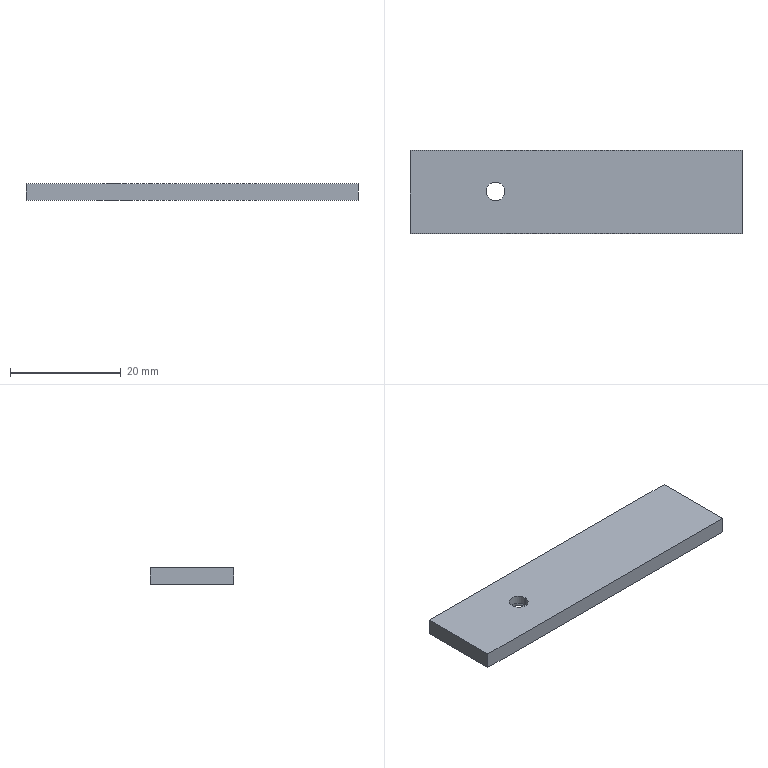Part | SolidWorks | features 3DProfileFeature 1, Extrusion 1, HoleWzd 1 | 1 solid | 10 faces | box 60 x 15 x 3 mm | volume 2658 mm3 | plane 6 | cone 2 | cylinder 2 | commonest cylinder face diameters 3.4 x2
STEP:
#1=CARTESIAN_POINT('',(-12.834,0.1148,1.45));
#2=VERTEX_POINT('',#1);
#3=CARTESIAN_POINT('',(-16.234,0.1148,1.45));
#4=VERTEX_POINT('',#3);
#5=CARTESIAN_POINT('',(-14.534,0.1148,1.45));
#6=DIRECTION('',(0.,0.,-1.));
#7=DIRECTION('',(-1.,0.,0.));
#8=AXIS2_PLACEMENT_3D('',#5,#6,#7);
#9=CIRCLE('',#8,1.7);
#10=EDGE_CURVE('',#2,#4,#9,.T.);
#11=ORIENTED_EDGE('',*,*,#10,.F.);
#12=CARTESIAN_POINT('',(-11.384,0.1148,0.));
#13=VERTEX_POINT('',#12);
#14=CARTESIAN_POINT('',(-11.384,0.1148,0.));
#15=DIRECTION('',(0.7071,0.,-0.7071));
#16=VECTOR('',#15,1000.);
#17=LINE('',#14,#16);
#18=EDGE_CURVE('',#2,#13,#17,.T.);
#19=ORIENTED_EDGE('',*,*,#18,.T.);
#20=CARTESIAN_POINT('',(-17.684,0.1148,0.));
#21=VERTEX_POINT('',#20);
#22=CARTESIAN_POINT('',(-14.534,0.1148,0.));
#23=DIRECTION('',(0.,0.,-1.));
#24=DIRECTION('',(-1.,0.,0.));
#25=AXIS2_PLACEMENT_3D('',#22,#23,#24);
#26=CIRCLE('',#25,3.15);
#27=EDGE_CURVE('',#13,#21,#26,.T.);
#28=ORIENTED_EDGE('',*,*,#27,.T.);
#29=CARTESIAN_POINT('',(-17.684,0.1148,0.));
#30=DIRECTION('',(-0.7071,0.,-0.7071));
#31=VECTOR('',#30,1000.);
#32=LINE('',#29,#31);
#33=EDGE_CURVE('',#4,#21,#32,.T.);
#34=ORIENTED_EDGE('',*,*,#33,.F.);
#35=EDGE_LOOP('',(#11,#19,#28,#34));
#36=FACE_OUTER_BOUND('',#35,.T.);
#37=CARTESIAN_POINT('',(-14.534,0.1148,0.));
#38=DIRECTION('',(0.,0.,-1.));
#39=DIRECTION('',(-1.,0.,0.));
#40=AXIS2_PLACEMENT_3D('',#37,#38,#39);
#41=CONICAL_SURFACE('',#40,3.15,0.7854);
#42=ADVANCED_FACE('',(#36),#41,.F.);
#43=CARTESIAN_POINT('',(-12.834,0.1148,3.));
#44=VERTEX_POINT('',#43);
#45=CARTESIAN_POINT('',(-16.234,0.1148,3.));
#46=VERTEX_POINT('',#45);
#47=CARTESIAN_POINT('',(-14.534,0.1148,3.));
#48=DIRECTION('',(0.,0.,-1.));
#49=DIRECTION('',(-1.,0.,0.));
#50=AXIS2_PLACEMENT_3D('',#47,#48,#49);
#51=CIRCLE('',#50,1.7);
#52=EDGE_CURVE('',#44,#46,#51,.T.);
#53=ORIENTED_EDGE('',*,*,#52,.F.);
#54=CARTESIAN_POINT('',(-12.834,0.1148,0.));
#55=DIRECTION('',(0.,0.,-1.));
#56=VECTOR('',#55,1000.);
#57=LINE('',#54,#56);
#58=EDGE_CURVE('',#44,#2,#57,.T.);
#59=ORIENTED_EDGE('',*,*,#58,.T.);
#60=ORIENTED_EDGE('',*,*,#10,.T.);
#61=CARTESIAN_POINT('',(-16.234,0.1148,0.));
#62=DIRECTION('',(0.,0.,-1.));
#63=VECTOR('',#62,1000.);
#64=LINE('',#61,#63);
#65=EDGE_CURVE('',#46,#4,#64,.T.);
#66=ORIENTED_EDGE('',*,*,#65,.F.);
#67=EDGE_LOOP('',(#53,#59,#60,#66));
#68=FACE_OUTER_BOUND('',#67,.T.);
#69=CARTESIAN_POINT('',(-14.534,0.1148,0.));
#70=DIRECTION('',(0.,0.,-1.));
#71=DIRECTION('',(-1.,0.,0.));
#72=AXIS2_PLACEMENT_3D('',#69,#70,#71);
#73=CYLINDRICAL_SURFACE('',#72,1.7);
#74=ADVANCED_FACE('',(#68),#73,.F.);
#75=CARTESIAN_POINT('',(30.,-7.5,0.));
#76=VERTEX_POINT('',#75);
#77=CARTESIAN_POINT('',(30.,7.5,0.));
#78=VERTEX_POINT('',#77);
#79=CARTESIAN_POINT('',(30.,-7.5,0.));
#80=DIRECTION('',(0.,1.,0.));
#81=VECTOR('',#80,1000.);
#82=LINE('',#79,#81);
#83=EDGE_CURVE('',#76,#78,#82,.T.);
#84=ORIENTED_EDGE('',*,*,#83,.T.);
#85=CARTESIAN_POINT('',(30.,7.5,3.));
#86=VERTEX_POINT('',#85);
#87=CARTESIAN_POINT('',(30.,7.5,3.));
#88=DIRECTION('',(0.,0.,-1.));
#89=VECTOR('',#88,1000.);
#90=LINE('',#87,#89);
#91=EDGE_CURVE('',#86,#78,#90,.T.);
#92=ORIENTED_EDGE('',*,*,#91,.F.);
#93=CARTESIAN_POINT('',(30.,-7.5,3.));
#94=VERTEX_POINT('',#93);
#95=CARTESIAN_POINT('',(30.,-7.5,3.));
#96=DIRECTION('',(0.,1.,0.));
#97=VECTOR('',#96,1000.);
#98=LINE('',#95,#97);
#99=EDGE_CURVE('',#94,#86,#98,.T.);
#100=ORIENTED_EDGE('',*,*,#99,.F.);
#101=CARTESIAN_POINT('',(30.,-7.5,3.));
#102=DIRECTION('',(0.,0.,-1.));
#103=VECTOR('',#102,1000.);
#104=LINE('',#101,#103);
#105=EDGE_CURVE('',#94,#76,#104,.T.);
#106=ORIENTED_EDGE('',*,*,#105,.T.);
#107=EDGE_LOOP('',(#84,#92,#100,#106));
#108=FACE_OUTER_BOUND('',#107,.T.);
#109=CARTESIAN_POINT('',(30.,-7.5,3.));
#110=DIRECTION('',(-1.,0.,0.));
#111=DIRECTION('',(0.,0.,1.));
#112=AXIS2_PLACEMENT_3D('',#109,#110,#111);
#113=PLANE('',#112);
#114=ADVANCED_FACE('',(#108),#113,.F.);
#115=CARTESIAN_POINT('',(-30.,7.5,0.));
#116=VERTEX_POINT('',#115);
#117=CARTESIAN_POINT('',(-30.,7.5,0.));
#118=DIRECTION('',(-1.,0.,0.));
#119=VECTOR('',#118,1000.);
#120=LINE('',#117,#119);
#121=EDGE_CURVE('',#78,#116,#120,.T.);
#122=ORIENTED_EDGE('',*,*,#121,.T.);
#123=CARTESIAN_POINT('',(-30.,7.5,3.));
#124=VERTEX_POINT('',#123);
#125=CARTESIAN_POINT('',(-30.,7.5,3.));
#126=DIRECTION('',(0.,0.,-1.));
#127=VECTOR('',#126,1000.);
#128=LINE('',#125,#127);
#129=EDGE_CURVE('',#124,#116,#128,.T.);
#130=ORIENTED_EDGE('',*,*,#129,.F.);
#131=CARTESIAN_POINT('',(-30.,7.5,3.));
#132=DIRECTION('',(-1.,0.,0.));
#133=VECTOR('',#132,1000.);
#134=LINE('',#131,#133);
#135=EDGE_CURVE('',#86,#124,#134,.T.);
#136=ORIENTED_EDGE('',*,*,#135,.F.);
#137=ORIENTED_EDGE('',*,*,#91,.T.);
#138=EDGE_LOOP('',(#122,#130,#136,#137));
#139=FACE_OUTER_BOUND('',#138,.T.);
#140=CARTESIAN_POINT('',(-30.,7.5,3.));
#141=DIRECTION('',(0.,-1.,0.));
#142=DIRECTION('',(0.,0.,-1.));
#143=AXIS2_PLACEMENT_3D('',#140,#141,#142);
#144=PLANE('',#143);
#145=ADVANCED_FACE('',(#139),#144,.F.);
#146=CARTESIAN_POINT('',(-30.,-7.5,0.));
#147=VERTEX_POINT('',#146);
#148=CARTESIAN_POINT('',(-30.,-7.5,0.));
#149=DIRECTION('',(0.,-1.,0.));
#150=VECTOR('',#149,1000.);
#151=LINE('',#148,#150);
#152=EDGE_CURVE('',#116,#147,#151,.T.);
#153=ORIENTED_EDGE('',*,*,#152,.T.);
#154=CARTESIAN_POINT('',(-30.,-7.5,3.));
#155=VERTEX_POINT('',#154);
#156=CARTESIAN_POINT('',(-30.,-7.5,3.));
#157=DIRECTION('',(0.,0.,-1.));
#158=VECTOR('',#157,1000.);
#159=LINE('',#156,#158);
#160=EDGE_CURVE('',#155,#147,#159,.T.);
#161=ORIENTED_EDGE('',*,*,#160,.F.);
#162=CARTESIAN_POINT('',(-30.,-7.5,3.));
#163=DIRECTION('',(0.,-1.,0.));
#164=VECTOR('',#163,1000.);
#165=LINE('',#162,#164);
#166=EDGE_CURVE('',#124,#155,#165,.T.);
#167=ORIENTED_EDGE('',*,*,#166,.F.);
#168=ORIENTED_EDGE('',*,*,#129,.T.);
#169=EDGE_LOOP('',(#153,#161,#167,#168));
#170=FACE_OUTER_BOUND('',#169,.T.);
#171=CARTESIAN_POINT('',(-30.,-7.5,3.));
#172=DIRECTION('',(1.,0.,0.));
#173=DIRECTION('',(0.,0.,-1.));
#174=AXIS2_PLACEMENT_3D('',#171,#172,#173);
#175=PLANE('',#174);
#176=ADVANCED_FACE('',(#170),#175,.F.);
#177=CARTESIAN_POINT('',(-30.,-7.5,0.));
#178=DIRECTION('',(1.,0.,0.));
#179=VECTOR('',#178,1000.);
#180=LINE('',#177,#179);
#181=EDGE_CURVE('',#147,#76,#180,.T.);
#182=ORIENTED_EDGE('',*,*,#181,.T.);
#183=ORIENTED_EDGE('',*,*,#105,.F.);
#184=CARTESIAN_POINT('',(-30.,-7.5,3.));
#185=DIRECTION('',(1.,0.,0.));
#186=VECTOR('',#185,1000.);
#187=LINE('',#184,#186);
#188=EDGE_CURVE('',#155,#94,#187,.T.);
#189=ORIENTED_EDGE('',*,*,#188,.F.);
#190=ORIENTED_EDGE('',*,*,#160,.T.);
#191=EDGE_LOOP('',(#182,#183,#189,#190));
#192=FACE_OUTER_BOUND('',#191,.T.);
#193=CARTESIAN_POINT('',(-30.,-7.5,3.));
#194=DIRECTION('',(0.,1.,0.));
#195=DIRECTION('',(0.,0.,1.));
#196=AXIS2_PLACEMENT_3D('',#193,#194,#195);
#197=PLANE('',#196);
#198=ADVANCED_FACE('',(#192),#197,.F.);
#199=CARTESIAN_POINT('',(-14.534,0.1148,3.));
#200=DIRECTION('',(0.,0.,-1.));
#201=DIRECTION('',(-1.,0.,0.));
#202=AXIS2_PLACEMENT_3D('',#199,#200,#201);
#203=CIRCLE('',#202,1.7);
#204=EDGE_CURVE('',#46,#44,#203,.T.);
#205=ORIENTED_EDGE('',*,*,#204,.T.);
#206=ORIENTED_EDGE('',*,*,#52,.T.);
#207=EDGE_LOOP('',(#205,#206));
#208=FACE_BOUND('',#207,.T.);
#209=ORIENTED_EDGE('',*,*,#99,.T.);
#210=ORIENTED_EDGE('',*,*,#135,.T.);
#211=ORIENTED_EDGE('',*,*,#166,.T.);
#212=ORIENTED_EDGE('',*,*,#188,.T.);
#213=EDGE_LOOP('',(#209,#210,#211,#212));
#214=FACE_OUTER_BOUND('',#213,.T.);
#215=CARTESIAN_POINT('',(0.,0.,3.));
#216=DIRECTION('',(0.,0.,-1.));
#217=DIRECTION('',(-1.,0.,0.));
#218=AXIS2_PLACEMENT_3D('',#215,#216,#217);
#219=PLANE('',#218);
#220=ADVANCED_FACE('',(#208,#214),#219,.F.);
#221=CARTESIAN_POINT('',(-14.534,0.1148,0.));
#222=DIRECTION('',(0.,0.,-1.));
#223=DIRECTION('',(-1.,0.,0.));
#224=AXIS2_PLACEMENT_3D('',#221,#222,#223);
#225=CIRCLE('',#224,3.15);
#226=EDGE_CURVE('',#21,#13,#225,.T.);
#227=ORIENTED_EDGE('',*,*,#226,.F.);
#228=ORIENTED_EDGE('',*,*,#27,.F.);
#229=EDGE_LOOP('',(#227,#228));
#230=FACE_BOUND('',#229,.T.);
#231=ORIENTED_EDGE('',*,*,#83,.F.);
#232=ORIENTED_EDGE('',*,*,#181,.F.);
#233=ORIENTED_EDGE('',*,*,#152,.F.);
#234=ORIENTED_EDGE('',*,*,#121,.F.);
#235=EDGE_LOOP('',(#231,#232,#233,#234));
#236=FACE_OUTER_BOUND('',#235,.T.);
#237=CARTESIAN_POINT('',(0.,0.,0.));
#238=DIRECTION('',(0.,0.,-1.));
#239=DIRECTION('',(-1.,0.,0.));
#240=AXIS2_PLACEMENT_3D('',#237,#238,#239);
#241=PLANE('',#240);
#242=ADVANCED_FACE('',(#230,#236),#241,.T.);
#243=ORIENTED_EDGE('',*,*,#58,.F.);
#244=ORIENTED_EDGE('',*,*,#204,.F.);
#245=ORIENTED_EDGE('',*,*,#65,.T.);
#246=CARTESIAN_POINT('',(-14.534,0.1148,1.45));
#247=DIRECTION('',(0.,0.,-1.));
#248=DIRECTION('',(-1.,0.,0.));
#249=AXIS2_PLACEMENT_3D('',#246,#247,#248);
#250=CIRCLE('',#249,1.7);
#251=EDGE_CURVE('',#4,#2,#250,.T.);
#252=ORIENTED_EDGE('',*,*,#251,.T.);
#253=EDGE_LOOP('',(#243,#244,#245,#252));
#254=FACE_OUTER_BOUND('',#253,.T.);
#255=CARTESIAN_POINT('',(-14.534,0.1148,0.));
#256=DIRECTION('',(0.,0.,-1.));
#257=DIRECTION('',(-1.,0.,0.));
#258=AXIS2_PLACEMENT_3D('',#255,#256,#257);
#259=CYLINDRICAL_SURFACE('',#258,1.7);
#260=ADVANCED_FACE('',(#254),#259,.F.);
#261=ORIENTED_EDGE('',*,*,#18,.F.);
#262=ORIENTED_EDGE('',*,*,#251,.F.);
#263=ORIENTED_EDGE('',*,*,#33,.T.);
#264=ORIENTED_EDGE('',*,*,#226,.T.);
#265=EDGE_LOOP('',(#261,#262,#263,#264));
#266=FACE_OUTER_BOUND('',#265,.T.);
#267=CARTESIAN_POINT('',(-14.534,0.1148,0.));
#268=DIRECTION('',(0.,0.,-1.));
#269=DIRECTION('',(-1.,0.,0.));
#270=AXIS2_PLACEMENT_3D('',#267,#268,#269);
#271=CONICAL_SURFACE('',#270,3.15,0.7854);
#272=ADVANCED_FACE('',(#266),#271,.F.);
#273=CLOSED_SHELL('',(#42,#74,#114,#145,#176,#198,#220,#242,#260,#272));
#274=MANIFOLD_SOLID_BREP('',#273);
#275=CARTESIAN_POINT('',(0.,0.,0.));
#276=DIRECTION('',(0.,0.,1.));
#277=DIRECTION('',(1.,0.,0.));
#278=AXIS2_PLACEMENT_3D('',#275,#276,#277);
#279=(LENGTH_UNIT()NAMED_UNIT(*)SI_UNIT(.MILLI.,.METRE.));
#280=UNCERTAINTY_MEASURE_WITH_UNIT(LENGTH_MEASURE(0.00001),#279,'','');
#281=(NAMED_UNIT(*)PLANE_ANGLE_UNIT()SI_UNIT($,.RADIAN.));
#282=(NAMED_UNIT(*)SI_UNIT($,.STERADIAN.)SOLID_ANGLE_UNIT());
#283=(GEOMETRIC_REPRESENTATION_CONTEXT(3)GLOBAL_UNCERTAINTY_ASSIGNED_CONTEXT((#280))GLOBAL_UNIT_ASSIGNED_CONTEXT((#279,#281,#282))REPRESENTATION_CONTEXT('',''));
#284=ADVANCED_BREP_SHAPE_REPRESENTATION('',(#274,#278),#283);